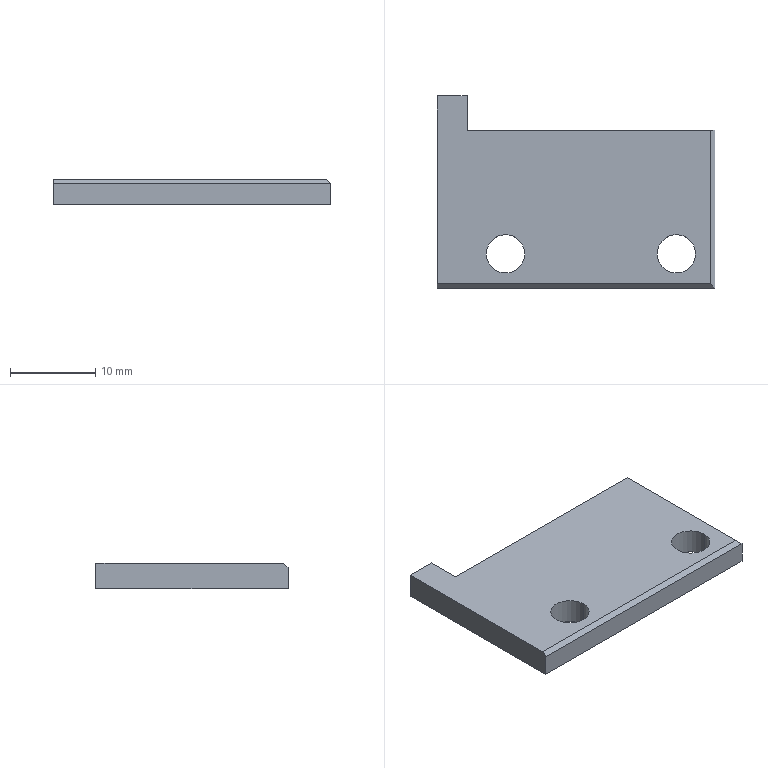Part | NX | 1 solid | 14 faces | box 32.5 x 22.5 x 3 mm | volume 1744 mm3 | plane 10 | cylinder 4 | commonest cylinder face diameters 4.5 x4
STEP:
#1=CARTESIAN_POINT('',(4.5,0.,1.));
#2=VERTEX_POINT('',#1);
#3=CARTESIAN_POINT('',(4.5,-22.5,1.));
#4=VERTEX_POINT('',#3);
#5=CARTESIAN_POINT('',(4.5,0.,1.));
#6=DIRECTION('',(0.,-1.,0.));
#7=VECTOR('',#6,1000.);
#8=LINE('',#5,#7);
#9=EDGE_CURVE('',#2,#4,#8,.T.);
#10=ORIENTED_EDGE('',*,*,#9,.F.);
#11=CARTESIAN_POINT('',(8.,0.,1.));
#12=VERTEX_POINT('',#11);
#13=CARTESIAN_POINT('',(0.,0.,1.));
#14=DIRECTION('',(1.,0.,0.));
#15=VECTOR('',#14,1000.);
#16=LINE('',#13,#15);
#17=EDGE_CURVE('',#2,#12,#16,.T.);
#18=ORIENTED_EDGE('',*,*,#17,.T.);
#19=CARTESIAN_POINT('',(8.,-4.,1.));
#20=VERTEX_POINT('',#19);
#21=CARTESIAN_POINT('',(8.,0.,1.));
#22=DIRECTION('',(0.,1.,0.));
#23=VECTOR('',#22,1000.);
#24=LINE('',#21,#23);
#25=EDGE_CURVE('',#20,#12,#24,.T.);
#26=ORIENTED_EDGE('',*,*,#25,.F.);
#27=CARTESIAN_POINT('',(37.,-4.,1.));
#28=VERTEX_POINT('',#27);
#29=CARTESIAN_POINT('',(0.,-4.,1.));
#30=DIRECTION('',(-1.,0.,0.));
#31=VECTOR('',#30,1000.);
#32=LINE('',#29,#31);
#33=EDGE_CURVE('',#28,#20,#32,.T.);
#34=ORIENTED_EDGE('',*,*,#33,.F.);
#35=CARTESIAN_POINT('',(37.,-22.5,1.));
#36=VERTEX_POINT('',#35);
#37=CARTESIAN_POINT('',(37.,0.,1.));
#38=DIRECTION('',(0.,-1.,0.));
#39=VECTOR('',#38,1000.);
#40=LINE('',#37,#39);
#41=EDGE_CURVE('',#28,#36,#40,.T.);
#42=ORIENTED_EDGE('',*,*,#41,.T.);
#43=CARTESIAN_POINT('',(0.,-22.5,1.));
#44=DIRECTION('',(-1.,0.,0.));
#45=VECTOR('',#44,1000.);
#46=LINE('',#43,#45);
#47=EDGE_CURVE('',#36,#4,#46,.T.);
#48=ORIENTED_EDGE('',*,*,#47,.T.);
#49=EDGE_LOOP('',(#10,#18,#26,#34,#42,#48));
#50=FACE_BOUND('',#49,.T.);
#51=CARTESIAN_POINT('',(34.75,-18.5,1.));
#52=VERTEX_POINT('',#51);
#53=CARTESIAN_POINT('',(30.25,-18.5,1.));
#54=VERTEX_POINT('',#53);
#55=CARTESIAN_POINT('',(32.5,-18.5,1.));
#56=DIRECTION('',(0.,0.,-1.));
#57=DIRECTION('',(-1.,0.,0.));
#58=AXIS2_PLACEMENT_3D('',#55,#56,#57);
#59=CIRCLE('',#58,2.25);
#60=EDGE_CURVE('',#52,#54,#59,.T.);
#61=ORIENTED_EDGE('',*,*,#60,.F.);
#62=CARTESIAN_POINT('',(32.5,-18.5,1.));
#63=DIRECTION('',(0.,0.,-1.));
#64=DIRECTION('',(-1.,0.,0.));
#65=AXIS2_PLACEMENT_3D('',#62,#63,#64);
#66=CIRCLE('',#65,2.25);
#67=EDGE_CURVE('',#54,#52,#66,.T.);
#68=ORIENTED_EDGE('',*,*,#67,.F.);
#69=EDGE_LOOP('',(#61,#68));
#70=FACE_BOUND('',#69,.T.);
#71=CARTESIAN_POINT('',(10.25,-18.5,1.));
#72=VERTEX_POINT('',#71);
#73=CARTESIAN_POINT('',(14.75,-18.5,1.));
#74=VERTEX_POINT('',#73);
#75=CARTESIAN_POINT('',(12.5,-18.5,1.));
#76=DIRECTION('',(0.,0.,-1.));
#77=DIRECTION('',(-1.,0.,0.));
#78=AXIS2_PLACEMENT_3D('',#75,#76,#77);
#79=CIRCLE('',#78,2.25);
#80=EDGE_CURVE('',#72,#74,#79,.T.);
#81=ORIENTED_EDGE('',*,*,#80,.F.);
#82=CARTESIAN_POINT('',(12.5,-18.5,1.));
#83=DIRECTION('',(0.,0.,-1.));
#84=DIRECTION('',(-1.,0.,0.));
#85=AXIS2_PLACEMENT_3D('',#82,#83,#84);
#86=CIRCLE('',#85,2.25);
#87=EDGE_CURVE('',#74,#72,#86,.T.);
#88=ORIENTED_EDGE('',*,*,#87,.F.);
#89=EDGE_LOOP('',(#81,#88));
#90=FACE_BOUND('',#89,.T.);
#91=CARTESIAN_POINT('',(32.,0.,1.));
#92=DIRECTION('',(0.,0.,1.));
#93=DIRECTION('',(1.,0.,0.));
#94=AXIS2_PLACEMENT_3D('',#91,#92,#93);
#95=PLANE('',#94);
#96=ADVANCED_FACE('',(#50,#70,#90),#95,.F.);
#97=CARTESIAN_POINT('',(36.5,-22.,4.));
#98=VERTEX_POINT('',#97);
#99=CARTESIAN_POINT('',(4.5,-22.,4.));
#100=VERTEX_POINT('',#99);
#101=CARTESIAN_POINT('',(0.,-22.,4.));
#102=DIRECTION('',(-1.,0.,0.));
#103=VECTOR('',#102,1000.);
#104=LINE('',#101,#103);
#105=EDGE_CURVE('',#98,#100,#104,.T.);
#106=ORIENTED_EDGE('',*,*,#105,.T.);
#107=CARTESIAN_POINT('',(4.5,-22.5,3.5));
#108=VERTEX_POINT('',#107);
#109=CARTESIAN_POINT('',(4.5,-26.,0.));
#110=DIRECTION('',(0.,-0.7071,-0.7071));
#111=VECTOR('',#110,1000.);
#112=LINE('',#109,#111);
#113=EDGE_CURVE('',#100,#108,#112,.T.);
#114=ORIENTED_EDGE('',*,*,#113,.T.);
#115=CARTESIAN_POINT('',(37.,-22.5,3.5));
#116=VERTEX_POINT('',#115);
#117=CARTESIAN_POINT('',(0.,-22.5,3.5));
#118=DIRECTION('',(-1.,0.,0.));
#119=VECTOR('',#118,1000.);
#120=LINE('',#117,#119);
#121=EDGE_CURVE('',#116,#108,#120,.T.);
#122=ORIENTED_EDGE('',*,*,#121,.F.);
#123=CARTESIAN_POINT('',(40.5,-26.,0.));
#124=DIRECTION('',(0.5774,-0.5774,-0.5774));
#125=VECTOR('',#124,1000.);
#126=LINE('',#123,#125);
#127=EDGE_CURVE('',#98,#116,#126,.T.);
#128=ORIENTED_EDGE('',*,*,#127,.F.);
#129=EDGE_LOOP('',(#106,#114,#122,#128));
#130=FACE_BOUND('',#129,.T.);
#131=CARTESIAN_POINT('',(17.25,-22.25,3.75));
#132=DIRECTION('',(0.,-0.7071,0.7071));
#133=DIRECTION('',(-1.,0.,0.));
#134=AXIS2_PLACEMENT_3D('',#131,#132,#133);
#135=PLANE('',#134);
#136=ADVANCED_FACE('',(#130),#135,.T.);
#137=CARTESIAN_POINT('',(37.,-4.,3.5));
#138=VERTEX_POINT('',#137);
#139=CARTESIAN_POINT('',(37.,0.,3.5));
#140=DIRECTION('',(0.,-1.,0.));
#141=VECTOR('',#140,1000.);
#142=LINE('',#139,#141);
#143=EDGE_CURVE('',#138,#116,#142,.T.);
#144=ORIENTED_EDGE('',*,*,#143,.T.);
#145=CARTESIAN_POINT('',(37.,-22.5,0.));
#146=DIRECTION('',(0.,0.,-1.));
#147=VECTOR('',#146,1000.);
#148=LINE('',#145,#147);
#149=EDGE_CURVE('',#116,#36,#148,.T.);
#150=ORIENTED_EDGE('',*,*,#149,.T.);
#151=ORIENTED_EDGE('',*,*,#41,.F.);
#152=CARTESIAN_POINT('',(37.,-4.,0.));
#153=DIRECTION('',(0.,0.,-1.));
#154=VECTOR('',#153,1000.);
#155=LINE('',#152,#154);
#156=EDGE_CURVE('',#138,#28,#155,.T.);
#157=ORIENTED_EDGE('',*,*,#156,.F.);
#158=EDGE_LOOP('',(#144,#150,#151,#157));
#159=FACE_BOUND('',#158,.T.);
#160=CARTESIAN_POINT('',(37.,-22.5,0.));
#161=DIRECTION('',(1.,0.,0.));
#162=DIRECTION('',(0.,1.,0.));
#163=AXIS2_PLACEMENT_3D('',#160,#161,#162);
#164=PLANE('',#163);
#165=ADVANCED_FACE('',(#159),#164,.T.);
#166=ORIENTED_EDGE('',*,*,#105,.F.);
#167=CARTESIAN_POINT('',(36.5,-4.,4.));
#168=VERTEX_POINT('',#167);
#169=CARTESIAN_POINT('',(36.5,0.,4.));
#170=DIRECTION('',(0.,-1.,0.));
#171=VECTOR('',#170,1000.);
#172=LINE('',#169,#171);
#173=EDGE_CURVE('',#168,#98,#172,.T.);
#174=ORIENTED_EDGE('',*,*,#173,.F.);
#175=CARTESIAN_POINT('',(8.,-4.,4.));
#176=VERTEX_POINT('',#175);
#177=CARTESIAN_POINT('',(0.,-4.,4.));
#178=DIRECTION('',(-1.,0.,0.));
#179=VECTOR('',#178,1000.);
#180=LINE('',#177,#179);
#181=EDGE_CURVE('',#168,#176,#180,.T.);
#182=ORIENTED_EDGE('',*,*,#181,.T.);
#183=CARTESIAN_POINT('',(8.,0.,4.));
#184=VERTEX_POINT('',#183);
#185=CARTESIAN_POINT('',(8.,0.,4.));
#186=DIRECTION('',(0.,1.,0.));
#187=VECTOR('',#186,1000.);
#188=LINE('',#185,#187);
#189=EDGE_CURVE('',#176,#184,#188,.T.);
#190=ORIENTED_EDGE('',*,*,#189,.T.);
#191=CARTESIAN_POINT('',(4.5,0.,4.));
#192=VERTEX_POINT('',#191);
#193=CARTESIAN_POINT('',(0.,0.,4.));
#194=DIRECTION('',(1.,0.,0.));
#195=VECTOR('',#194,1000.);
#196=LINE('',#193,#195);
#197=EDGE_CURVE('',#192,#184,#196,.T.);
#198=ORIENTED_EDGE('',*,*,#197,.F.);
#199=CARTESIAN_POINT('',(4.5,0.,4.));
#200=DIRECTION('',(0.,-1.,0.));
#201=VECTOR('',#200,1000.);
#202=LINE('',#199,#201);
#203=EDGE_CURVE('',#192,#100,#202,.T.);
#204=ORIENTED_EDGE('',*,*,#203,.T.);
#205=EDGE_LOOP('',(#166,#174,#182,#190,#198,#204));
#206=FACE_BOUND('',#205,.T.);
#207=CARTESIAN_POINT('',(14.75,-18.5,4.));
#208=VERTEX_POINT('',#207);
#209=CARTESIAN_POINT('',(10.25,-18.5,4.));
#210=VERTEX_POINT('',#209);
#211=CARTESIAN_POINT('',(12.5,-18.5,4.));
#212=DIRECTION('',(0.,0.,-1.));
#213=DIRECTION('',(-1.,0.,0.));
#214=AXIS2_PLACEMENT_3D('',#211,#212,#213);
#215=CIRCLE('',#214,2.25);
#216=EDGE_CURVE('',#208,#210,#215,.T.);
#217=ORIENTED_EDGE('',*,*,#216,.T.);
#218=CARTESIAN_POINT('',(12.5,-18.5,4.));
#219=DIRECTION('',(0.,0.,-1.));
#220=DIRECTION('',(-1.,0.,0.));
#221=AXIS2_PLACEMENT_3D('',#218,#219,#220);
#222=CIRCLE('',#221,2.25);
#223=EDGE_CURVE('',#210,#208,#222,.T.);
#224=ORIENTED_EDGE('',*,*,#223,.T.);
#225=EDGE_LOOP('',(#217,#224));
#226=FACE_BOUND('',#225,.T.);
#227=CARTESIAN_POINT('',(30.25,-18.5,4.));
#228=VERTEX_POINT('',#227);
#229=CARTESIAN_POINT('',(34.75,-18.5,4.));
#230=VERTEX_POINT('',#229);
#231=CARTESIAN_POINT('',(32.5,-18.5,4.));
#232=DIRECTION('',(0.,0.,-1.));
#233=DIRECTION('',(-1.,0.,0.));
#234=AXIS2_PLACEMENT_3D('',#231,#232,#233);
#235=CIRCLE('',#234,2.25);
#236=EDGE_CURVE('',#228,#230,#235,.T.);
#237=ORIENTED_EDGE('',*,*,#236,.T.);
#238=CARTESIAN_POINT('',(32.5,-18.5,4.));
#239=DIRECTION('',(0.,0.,-1.));
#240=DIRECTION('',(-1.,0.,0.));
#241=AXIS2_PLACEMENT_3D('',#238,#239,#240);
#242=CIRCLE('',#241,2.25);
#243=EDGE_CURVE('',#230,#228,#242,.T.);
#244=ORIENTED_EDGE('',*,*,#243,.T.);
#245=EDGE_LOOP('',(#237,#244));
#246=FACE_BOUND('',#245,.T.);
#247=CARTESIAN_POINT('',(0.,0.,4.));
#248=DIRECTION('',(0.,0.,1.));
#249=DIRECTION('',(1.,0.,0.));
#250=AXIS2_PLACEMENT_3D('',#247,#248,#249);
#251=PLANE('',#250);
#252=ADVANCED_FACE('',(#206,#226,#246),#251,.T.);
#253=ORIENTED_EDGE('',*,*,#203,.F.);
#254=CARTESIAN_POINT('',(4.5,0.,0.));
#255=DIRECTION('',(0.,0.,1.));
#256=VECTOR('',#255,1000.);
#257=LINE('',#254,#256);
#258=EDGE_CURVE('',#2,#192,#257,.T.);
#259=ORIENTED_EDGE('',*,*,#258,.F.);
#260=ORIENTED_EDGE('',*,*,#9,.T.);
#261=CARTESIAN_POINT('',(4.5,-22.5,0.));
#262=DIRECTION('',(0.,0.,-1.));
#263=VECTOR('',#262,1000.);
#264=LINE('',#261,#263);
#265=EDGE_CURVE('',#108,#4,#264,.T.);
#266=ORIENTED_EDGE('',*,*,#265,.F.);
#267=ORIENTED_EDGE('',*,*,#113,.F.);
#268=EDGE_LOOP('',(#253,#259,#260,#266,#267));
#269=FACE_BOUND('',#268,.T.);
#270=CARTESIAN_POINT('',(4.5,-8.5,-11.));
#271=DIRECTION('',(1.,0.,0.));
#272=DIRECTION('',(0.,1.,0.));
#273=AXIS2_PLACEMENT_3D('',#270,#271,#272);
#274=PLANE('',#273);
#275=ADVANCED_FACE('',(#269),#274,.F.);
#276=ORIENTED_EDGE('',*,*,#197,.T.);
#277=CARTESIAN_POINT('',(8.,0.,0.));
#278=DIRECTION('',(0.,0.,-1.));
#279=VECTOR('',#278,1000.);
#280=LINE('',#277,#279);
#281=EDGE_CURVE('',#184,#12,#280,.T.);
#282=ORIENTED_EDGE('',*,*,#281,.T.);
#283=ORIENTED_EDGE('',*,*,#17,.F.);
#284=ORIENTED_EDGE('',*,*,#258,.T.);
#285=EDGE_LOOP('',(#276,#282,#283,#284));
#286=FACE_BOUND('',#285,.T.);
#287=CARTESIAN_POINT('',(32.,0.,0.));
#288=DIRECTION('',(0.,1.,0.));
#289=DIRECTION('',(1.,0.,0.));
#290=AXIS2_PLACEMENT_3D('',#287,#288,#289);
#291=PLANE('',#290);
#292=ADVANCED_FACE('',(#286),#291,.T.);
#293=ORIENTED_EDGE('',*,*,#25,.T.);
#294=ORIENTED_EDGE('',*,*,#281,.F.);
#295=ORIENTED_EDGE('',*,*,#189,.F.);
#296=CARTESIAN_POINT('',(8.,-4.,0.));
#297=DIRECTION('',(0.,0.,1.));
#298=VECTOR('',#297,1000.);
#299=LINE('',#296,#298);
#300=EDGE_CURVE('',#20,#176,#299,.T.);
#301=ORIENTED_EDGE('',*,*,#300,.F.);
#302=EDGE_LOOP('',(#293,#294,#295,#301));
#303=FACE_BOUND('',#302,.T.);
#304=CARTESIAN_POINT('',(8.,0.,5.));
#305=DIRECTION('',(-1.,0.,0.));
#306=DIRECTION('',(0.,0.,1.));
#307=AXIS2_PLACEMENT_3D('',#304,#305,#306);
#308=PLANE('',#307);
#309=ADVANCED_FACE('',(#303),#308,.F.);
#310=ORIENTED_EDGE('',*,*,#33,.T.);
#311=ORIENTED_EDGE('',*,*,#300,.T.);
#312=ORIENTED_EDGE('',*,*,#181,.F.);
#313=CARTESIAN_POINT('',(40.5,-4.,0.));
#314=DIRECTION('',(0.7071,0.,-0.7071));
#315=VECTOR('',#314,1000.);
#316=LINE('',#313,#315);
#317=EDGE_CURVE('',#168,#138,#316,.T.);
#318=ORIENTED_EDGE('',*,*,#317,.T.);
#319=ORIENTED_EDGE('',*,*,#156,.T.);
#320=EDGE_LOOP('',(#310,#311,#312,#318,#319));
#321=FACE_BOUND('',#320,.T.);
#322=CARTESIAN_POINT('',(3.,-4.,5.));
#323=DIRECTION('',(0.,-1.,0.));
#324=DIRECTION('',(0.,0.,-1.));
#325=AXIS2_PLACEMENT_3D('',#322,#323,#324);
#326=PLANE('',#325);
#327=ADVANCED_FACE('',(#321),#326,.F.);
#328=ORIENTED_EDGE('',*,*,#216,.F.);
#329=CARTESIAN_POINT('',(14.75,-18.5,5.));
#330=DIRECTION('',(0.,0.,-1.));
#331=VECTOR('',#330,1000.);
#332=LINE('',#329,#331);
#333=EDGE_CURVE('',#208,#74,#332,.T.);
#334=ORIENTED_EDGE('',*,*,#333,.T.);
#335=ORIENTED_EDGE('',*,*,#87,.T.);
#336=CARTESIAN_POINT('',(10.25,-18.5,5.));
#337=DIRECTION('',(0.,0.,-1.));
#338=VECTOR('',#337,1000.);
#339=LINE('',#336,#338);
#340=EDGE_CURVE('',#210,#72,#339,.T.);
#341=ORIENTED_EDGE('',*,*,#340,.F.);
#342=EDGE_LOOP('',(#328,#334,#335,#341));
#343=FACE_BOUND('',#342,.T.);
#344=CARTESIAN_POINT('',(12.5,-18.5,5.));
#345=DIRECTION('',(0.,0.,-1.));
#346=DIRECTION('',(-1.,0.,0.));
#347=AXIS2_PLACEMENT_3D('',#344,#345,#346);
#348=CYLINDRICAL_SURFACE('',#347,2.25);
#349=ADVANCED_FACE('',(#343),#348,.F.);
#350=ORIENTED_EDGE('',*,*,#149,.F.);
#351=ORIENTED_EDGE('',*,*,#121,.T.);
#352=ORIENTED_EDGE('',*,*,#265,.T.);
#353=ORIENTED_EDGE('',*,*,#47,.F.);
#354=EDGE_LOOP('',(#350,#351,#352,#353));
#355=FACE_BOUND('',#354,.T.);
#356=CARTESIAN_POINT('',(0.,-22.5,0.));
#357=DIRECTION('',(0.,-1.,0.));
#358=DIRECTION('',(0.,0.,-1.));
#359=AXIS2_PLACEMENT_3D('',#356,#357,#358);
#360=PLANE('',#359);
#361=ADVANCED_FACE('',(#355),#360,.T.);
#362=ORIENTED_EDGE('',*,*,#127,.T.);
#363=ORIENTED_EDGE('',*,*,#143,.F.);
#364=ORIENTED_EDGE('',*,*,#317,.F.);
#365=ORIENTED_EDGE('',*,*,#173,.T.);
#366=EDGE_LOOP('',(#362,#363,#364,#365));
#367=FACE_BOUND('',#366,.T.);
#368=CARTESIAN_POINT('',(36.75,-13.25,3.75));
#369=DIRECTION('',(0.7071,0.,0.7071));
#370=DIRECTION('',(0.,-1.,0.));
#371=AXIS2_PLACEMENT_3D('',#368,#369,#370);
#372=PLANE('',#371);
#373=ADVANCED_FACE('',(#367),#372,.T.);
#374=ORIENTED_EDGE('',*,*,#236,.F.);
#375=CARTESIAN_POINT('',(30.25,-18.5,5.));
#376=DIRECTION('',(0.,0.,-1.));
#377=VECTOR('',#376,1000.);
#378=LINE('',#375,#377);
#379=EDGE_CURVE('',#54,#228,#378,.F.);
#380=ORIENTED_EDGE('',*,*,#379,.F.);
#381=ORIENTED_EDGE('',*,*,#67,.T.);
#382=CARTESIAN_POINT('',(34.75,-18.5,5.));
#383=DIRECTION('',(0.,0.,-1.));
#384=VECTOR('',#383,1000.);
#385=LINE('',#382,#384);
#386=EDGE_CURVE('',#52,#230,#385,.F.);
#387=ORIENTED_EDGE('',*,*,#386,.T.);
#388=EDGE_LOOP('',(#374,#380,#381,#387));
#389=FACE_BOUND('',#388,.T.);
#390=CARTESIAN_POINT('',(32.5,-18.5,5.));
#391=DIRECTION('',(0.,0.,-1.));
#392=DIRECTION('',(-1.,0.,0.));
#393=AXIS2_PLACEMENT_3D('',#390,#391,#392);
#394=CYLINDRICAL_SURFACE('',#393,2.25);
#395=ADVANCED_FACE('',(#389),#394,.F.);
#396=ORIENTED_EDGE('',*,*,#80,.T.);
#397=ORIENTED_EDGE('',*,*,#333,.F.);
#398=ORIENTED_EDGE('',*,*,#223,.F.);
#399=ORIENTED_EDGE('',*,*,#340,.T.);
#400=EDGE_LOOP('',(#396,#397,#398,#399));
#401=FACE_BOUND('',#400,.T.);
#402=CARTESIAN_POINT('',(12.5,-18.5,5.));
#403=DIRECTION('',(0.,0.,-1.));
#404=DIRECTION('',(-1.,0.,0.));
#405=AXIS2_PLACEMENT_3D('',#402,#403,#404);
#406=CYLINDRICAL_SURFACE('',#405,2.25);
#407=ADVANCED_FACE('',(#401),#406,.F.);
#408=ORIENTED_EDGE('',*,*,#60,.T.);
#409=ORIENTED_EDGE('',*,*,#379,.T.);
#410=ORIENTED_EDGE('',*,*,#243,.F.);
#411=ORIENTED_EDGE('',*,*,#386,.F.);
#412=EDGE_LOOP('',(#408,#409,#410,#411));
#413=FACE_BOUND('',#412,.T.);
#414=CARTESIAN_POINT('',(32.5,-18.5,5.));
#415=DIRECTION('',(0.,0.,-1.));
#416=DIRECTION('',(-1.,0.,0.));
#417=AXIS2_PLACEMENT_3D('',#414,#415,#416);
#418=CYLINDRICAL_SURFACE('',#417,2.25);
#419=ADVANCED_FACE('',(#413),#418,.F.);
#420=CLOSED_SHELL('',(#96,#136,#165,#252,#275,#292,#309,#327,#349,#361,#373,#395,#407,#419));
#421=MANIFOLD_SOLID_BREP('',#420);
#422=(LENGTH_UNIT()NAMED_UNIT(*)SI_UNIT(.MILLI.,.METRE.));
#423=UNCERTAINTY_MEASURE_WITH_UNIT(LENGTH_MEASURE(0.00001),#422,'','');
#424=(NAMED_UNIT(*)PLANE_ANGLE_UNIT()SI_UNIT($,.RADIAN.));
#425=(NAMED_UNIT(*)SI_UNIT($,.STERADIAN.)SOLID_ANGLE_UNIT());
#426=(GEOMETRIC_REPRESENTATION_CONTEXT(3)GLOBAL_UNCERTAINTY_ASSIGNED_CONTEXT((#423))GLOBAL_UNIT_ASSIGNED_CONTEXT((#422,#424,#425))REPRESENTATION_CONTEXT('',''));
#427=ADVANCED_BREP_SHAPE_REPRESENTATION('',(#421),#426);